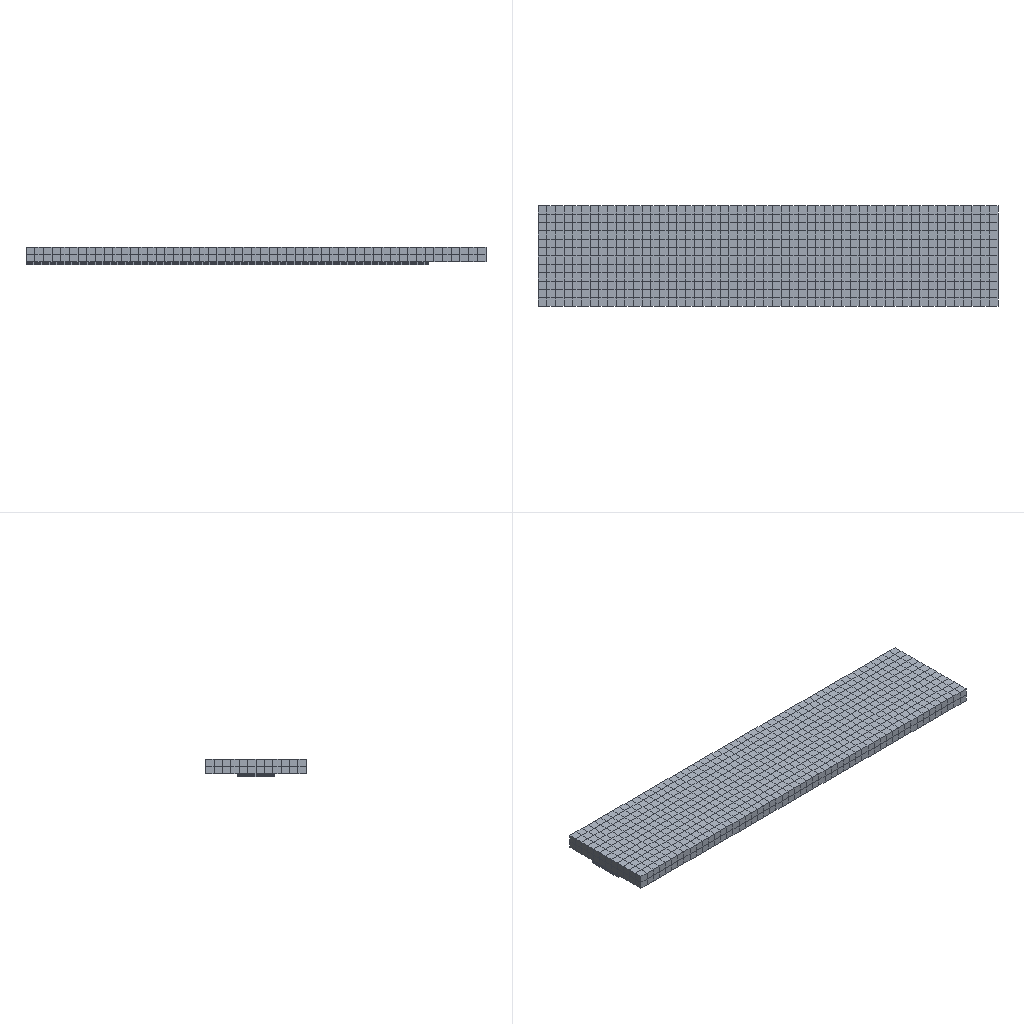Simulation study | abaqus
Set-up summary:
category,name,step,type,value,unit,region
solver,abaqus
solver,version,,,Abaqus/Standard 3DEXPERIENCE R2017x
units,not stated in the deck,,not stated
analysis,deck,,coupled temperature-displacement,coupled temperature-displacement
load_step,Step-1,Step-1,coupled temperature-displacement
load_step,Step-2,Step-2,coupled temperature-displacement
load_step,Step-3,Step-3,coupled temperature-displacement
load_step,Step-4,Step-4,coupled temperature-displacement
load_step,Step-5,Step-5,coupled temperature-displacement
load_step,Step-6,Step-6,coupled temperature-displacement
load_step,Step-7,Step-7,coupled temperature-displacement
load_step,Step-8,Step-8,coupled temperature-displacement
load_step,Step-9,Step-9,coupled temperature-displacement
load_step,Step-10,Step-10,coupled temperature-displacement
load_step,Step-11,Step-11,coupled temperature-displacement
load_step,Step-12,Step-12,coupled temperature-displacement
load_step,Step-13,Step-13,coupled temperature-displacement
load_step,Step-14,Step-14,coupled temperature-displacement
load_step,Step-15,Step-15,coupled temperature-displacement
load_step,Step-16,Step-16,coupled temperature-displacement
load_step,Step-17,Step-17,coupled temperature-displacement
load_step,requested,,,17
mesh,nodes,,,10058
mesh,elements,,,4632
element_type,C3D8T,,solid,4632
load,load commands in deck,,count,19
bc,support commands in deck,,count,1
material,AL,,in results
material,MATERIAL-1,,in results
check,setup vs results,,match,"per instance, exact: element labels, types and connectivity; labels of the nodes the elements use; coordinates of those nodes at SINGLE_PRECISION in 2 of 9 instance(s)"
Abaqus input file, long lists of numbers shortened:
*Heading
** Job name: Job-1 Model name: Model-1-Copy
** Generated by: Abaqus/CAE 2017
*Preprint, echo=NO, model=NO, history=NO, contact=NO
**
** PARTS
**
*Part, name=Part-1
*Node
      1,           0.,         -35.,           5.
      2,           0.,  -32.083,           5.
** (2104 more lines like these left out)
*Element, type=C3D8T
   1,   40,   41,   54,   53,    1,    2,   15,   14
   2,   41,   42,   55,   54,    2,    3,   16,   15
** (1270 more lines like these left out)
*Nset, nset=Set-4, generate
    1,  2106,     1
*Elset, elset=Set-4, generate
    1,  1272,     1
** Section: al
*Solid Section, elset=Set-4, material=al
,
*End Part
**
*Part, name=add
*Node
      1,   30.751,         -10.,           0.
      2,   30.751,         -10.,        0.125
** (992 more lines like these left out)
*Element, type=C3D8T
  1, 161, 166, 485, 315,   1,   2,  17,  84
  2, 315, 485, 486, 316,  84,  17,  18,  83
** (418 more lines like these left out)
*Nset, nset=Set-1, generate
   1,  994,    1
*Elset, elset=Set-1, generate
   1,  420,    1
*Orientation, name=Ori-1
1., 0., 0., 0., 1., 0.
1, 0.
** Section: com
*Solid Section, elset=Set-1, orientation=Ori-1, material=Material-1
,
*End Part
**
**
** ASSEMBLY
**
*Assembly, name=Assembly
**
*Instance, name=Part-1-1, part=Part-1
*End Instance
**
*Instance, name=add-1, part=add
         80.,     6.901,       -0.125
         80.,     6.901,       -0.125,          80.,     6.901,       -1.125,          90.
*End Instance
**
*Instance, name=add-1-lin-2-1, part=add
         80.,     6.901,        -0.25
         80.,     6.901,        -0.25,          80.,     6.901,        -1.25,          90.
*End Instance
**
*Instance, name=add-1-lin-3-1, part=add
         80.,     6.901,       -0.375
         80.,     6.901,       -0.375,          80.,     6.901,       -1.375,          90.
*End Instance
**
*Instance, name=add-1-lin-4-1, part=add
         80.,     6.901,         -0.5
         80.,     6.901,         -0.5,          80.,     6.901,         -1.5,          90.
*End Instance
**
*Instance, name=add-1-lin-5-1, part=add
         80.,     6.901,       -0.625
         80.,     6.901,       -0.625,          80.,     6.901,       -1.625,          90.
*End Instance
**
*Instance, name=add-1-lin-6-1, part=add
         80.,     6.901,        -0.75
         80.,     6.901,        -0.75,          80.,     6.901,        -1.75,          90.
*End Instance
**
*Instance, name=add-1-lin-7-1, part=add
         80.,     6.901,       -0.875
         80.,     6.901,       -0.875,          80.,     6.901,       -1.875,          90.
*End Instance
**
*Instance, name=add-1-lin-8-1, part=add
         80.,     6.901,          -1.
         80.,     6.901,          -1.,          80.,     6.901,          -2.,          90.
*End Instance
**
*Node
      1,           0.,        -17.5,       -0.125
*Node
      2,           0.,        -17.5,       -0.375
*Node
      3,           0.,        -17.5,       -0.625
*Node
      4,           0.,        -17.5,       -0.875
*Node
      5,         140.,        -17.5,        -0.25
*Node
      6,         140.,        -17.5,         -0.5
*Node
      7,         140.,        -17.5,        -0.75
*Nset, nset=Set-10, instance=Part-1-1, generate
 2068,  2106,     1
*Elset, elset=Set-10, instance=Part-1-1, generate
 1249,  1272,     1
*Nset, nset=Set-11, instance=Part-1-1
    1,    2,    3,    4,    5,    6,    7,    8,    9,   10,   11,   12,   13,   14,   15,   16
   17,   18,   19,   20,   21,   22,   23,   24,   25,   26,   27,   28,   29,   30,   31,   32
** (3 more lines like these left out)
*Elset, elset=Set-11, instance=Part-1-1
    1,    2,    3,    4,    5,    6,    7,    8,    9,   10,   11,   12,   13,   14,   15,   16
   17,   18,   19,   20,   21,   22,   23,   24, 1249, 1250, 1251, 1252, 1253, 1254, 1255, 1256
** (1 more lines like these left out)
*Nset, nset=Set-12, instance=Part-1-1, generate
    1,  2106,     1
*Nset, nset=Set-12, instance=add-1, generate
   1,  994,    1
*Nset, nset=Set-12, instance=add-1-lin-2-1, generate
   1,  994,    1
*Nset, nset=Set-12, instance=add-1-lin-6-1, generate
   1,  994,    1
*Nset, nset=Set-12, instance=add-1-lin-4-1, generate
   1,  994,    1
*Nset, nset=Set-12, instance=add-1-lin-8-1, generate
   1,  994,    1
*Nset, nset=Set-12, instance=add-1-lin-3-1, generate
   1,  994,    1
*Nset, nset=Set-12, instance=add-1-lin-7-1, generate
   1,  994,    1
*Nset, nset=Set-12, instance=add-1-lin-5-1, generate
   1,  994,    1
*Elset, elset=Set-12, instance=Part-1-1, generate
    1,  1272,     1
*Elset, elset=Set-12, instance=add-1, generate
   1,  420,    1
*Elset, elset=Set-12, instance=add-1-lin-2-1, generate
   1,  420,    1
*Elset, elset=Set-12, instance=add-1-lin-6-1, generate
   1,  420,    1
*Elset, elset=Set-12, instance=add-1-lin-4-1, generate
   1,  420,    1
*Elset, elset=Set-12, instance=add-1-lin-8-1, generate
   1,  420,    1
*Elset, elset=Set-12, instance=add-1-lin-3-1, generate
   1,  420,    1
*Elset, elset=Set-12, instance=add-1-lin-7-1, generate
   1,  420,    1
*Elset, elset=Set-12, instance=add-1-lin-5-1, generate
   1,  420,    1
*Nset, nset=Set-13, instance=Part-1-1, generate
    1,  2106,     1
*Nset, nset=Set-13, instance=add-1, generate
   1,  994,    1
*Nset, nset=Set-13, instance=add-1-lin-2-1, generate
   1,  994,    1
*Nset, nset=Set-13, instance=add-1-lin-6-1, generate
   1,  994,    1
*Nset, nset=Set-13, instance=add-1-lin-4-1, generate
   1,  994,    1
*Nset, nset=Set-13, instance=add-1-lin-8-1, generate
   1,  994,    1
*Nset, nset=Set-13, instance=add-1-lin-3-1, generate
   1,  994,    1
*Nset, nset=Set-13, instance=add-1-lin-7-1, generate
   1,  994,    1
*Nset, nset=Set-13, instance=add-1-lin-5-1, generate
   1,  994,    1
*Elset, elset=Set-13, instance=Part-1-1, generate
    1,  1272,     1
*Elset, elset=Set-13, instance=add-1, generate
   1,  420,    1
*Elset, elset=Set-13, instance=add-1-lin-2-1, generate
   1,  420,    1
*Elset, elset=Set-13, instance=add-1-lin-6-1, generate
   1,  420,    1
*Elset, elset=Set-13, instance=add-1-lin-4-1, generate
   1,  420,    1
*Elset, elset=Set-13, instance=add-1-lin-8-1, generate
   1,  420,    1
*Elset, elset=Set-13, instance=add-1-lin-3-1, generate
   1,  420,    1
*Elset, elset=Set-13, instance=add-1-lin-7-1, generate
   1,  420,    1
*Elset, elset=Set-13, instance=add-1-lin-5-1, generate
   1,  420,    1
*Nset, nset=Set-14, instance=add-1, generate
   1,  994,    1
*Nset, nset=Set-14, instance=add-1-lin-2-1, generate
   1,  994,    1
*Nset, nset=Set-14, instance=add-1-lin-4-1, generate
   1,  994,    1
*Nset, nset=Set-14, instance=add-1-lin-6-1, generate
   1,  994,    1
*Nset, nset=Set-14, instance=add-1-lin-8-1, generate
   1,  994,    1
*Nset, nset=Set-14, instance=add-1-lin-3-1, generate
   1,  994,    1
*Nset, nset=Set-14, instance=add-1-lin-7-1, generate
   1,  994,    1
*Nset, nset=Set-14, instance=add-1-lin-5-1, generate
   1,  994,    1
*Elset, elset=Set-14, instance=add-1, generate
   1,  420,    1
*Elset, elset=Set-14, instance=add-1-lin-2-1, generate
   1,  420,    1
*Elset, elset=Set-14, instance=add-1-lin-4-1, generate
   1,  420,    1
*Elset, elset=Set-14, instance=add-1-lin-6-1, generate
   1,  420,    1
*Elset, elset=Set-14, instance=add-1-lin-8-1, generate
   1,  420,    1
*Elset, elset=Set-14, instance=add-1-lin-3-1, generate
   1,  420,    1
*Elset, elset=Set-14, instance=add-1-lin-7-1, generate
   1,  420,    1
*Elset, elset=Set-14, instance=add-1-lin-5-1, generate
   1,  420,    1
*Nset, nset=Set-15, instance=add-1, generate
   1,  994,    1
*Elset, elset=Set-15, instance=add-1, generate
   1,  420,    1
*Nset, nset=Set-16, instance=add-1-lin-2-1, generate
   1,  994,    1
*Elset, elset=Set-16, instance=add-1-lin-2-1, generate
   1,  420,    1
*Nset, nset=Set-17, instance=add-1-lin-3-1, generate
   1,  994,    1
*Elset, elset=Set-17, instance=add-1-lin-3-1, generate
   1,  420,    1
*Nset, nset=Set-18, instance=add-1-lin-4-1, generate
   1,  994,    1
*Elset, elset=Set-18, instance=add-1-lin-4-1, generate
   1,  420,    1
*Nset, nset=Set-19, instance=add-1-lin-5-1, generate
   1,  994,    1
*Elset, elset=Set-19, instance=add-1-lin-5-1, generate
   1,  420,    1
*Nset, nset=Set-20, instance=add-1-lin-6-1, generate
   1,  994,    1
*Elset, elset=Set-20, instance=add-1-lin-6-1, generate
   1,  420,    1
*Nset, nset=Set-21, instance=add-1-lin-7-1, generate
   1,  994,    1
*Elset, elset=Set-21, instance=add-1-lin-7-1, generate
   1,  420,    1
*Nset, nset=Set-22, instance=add-1-lin-8-1, generate
   1,  994,    1
*Elset, elset=Set-22, instance=add-1-lin-8-1, generate
   1,  420,    1
*Nset, nset=Set-23, instance=add-1, generate
   1,  994,    1
*Nset, nset=Set-23, instance=add-1-lin-2-1, generate
   1,  994,    1
*Nset, nset=Set-23, instance=add-1-lin-4-1, generate
   1,  994,    1
*Nset, nset=Set-23, instance=add-1-lin-6-1, generate
   1,  994,    1
*Nset, nset=Set-23, instance=add-1-lin-8-1, generate
   1,  994,    1
*Nset, nset=Set-23, instance=add-1-lin-3-1, generate
   1,  994,    1
*Nset, nset=Set-23, instance=add-1-lin-7-1, generate
   1,  994,    1
*Nset, nset=Set-23, instance=add-1-lin-5-1, generate
   1,  994,    1
*Elset, elset=Set-23, instance=add-1, generate
   1,  420,    1
*Elset, elset=Set-23, instance=add-1-lin-2-1, generate
   1,  420,    1
*Elset, elset=Set-23, instance=add-1-lin-4-1, generate
   1,  420,    1
*Elset, elset=Set-23, instance=add-1-lin-6-1, generate
   1,  420,    1
*Elset, elset=Set-23, instance=add-1-lin-8-1, generate
   1,  420,    1
*Elset, elset=Set-23, instance=add-1-lin-3-1, generate
   1,  420,    1
*Elset, elset=Set-23, instance=add-1-lin-7-1, generate
   1,  420,    1
*Elset, elset=Set-23, instance=add-1-lin-5-1, generate
   1,  420,    1
*Elset, elset=_Surf-17_S6, internal, instance=add-1, generate
   1,  210,    1
*Surface, type=ELEMENT, name=Surf-17
_Surf-17_S6, S6
*Elset, elset=_Surf-18_S4, internal, instance=add-1, generate
 211,  420,    1
*Surface, type=ELEMENT, name=Surf-18
_Surf-18_S4, S4
*Elset, elset=_Surf-19_S6, internal, instance=add-1-lin-2-1, generate
   1,  210,    1
*Surface, type=ELEMENT, name=Surf-19
_Surf-19_S6, S6
*Elset, elset=_Surf-20_S4, internal, instance=add-1-lin-2-1, generate
 211,  420,    1
*Surface, type=ELEMENT, name=Surf-20
_Surf-20_S4, S4
*Elset, elset=_Surf-21_S4, internal, instance=add-1-lin-2-1, generate
 211,  420,    1
*Surface, type=ELEMENT, name=Surf-21
_Surf-21_S4, S4
*Elset, elset=_Surf-22_S6, internal, instance=add-1-lin-2-1, generate
   1,  210,    1
*Surface, type=ELEMENT, name=Surf-22
_Surf-22_S6, S6
*Elset, elset=_Surf-23_S6, internal, instance=add-1-lin-3-1, generate
   1,  210,    1
*Surface, type=ELEMENT, name=Surf-23
_Surf-23_S6, S6
*Elset, elset=_Surf-24_S4, internal, instance=add-1-lin-3-1, generate
 211,  420,    1
*Surface, type=ELEMENT, name=Surf-24
_Surf-24_S4, S4
*Elset, elset=_Surf-25_S6, internal, instance=add-1-lin-4-1, generate
   1,  210,    1
*Surface, type=ELEMENT, name=Surf-25
_Surf-25_S6, S6
*Elset, elset=_Surf-26_S4, internal, instance=add-1-lin-4-1, generate
 211,  420,    1
*Surface, type=ELEMENT, name=Surf-26
_Surf-26_S4, S4
*Elset, elset=_Surf-27_S6, internal, instance=add-1-lin-4-1, generate
   1,  210,    1
*Surface, type=ELEMENT, name=Surf-27
_Surf-27_S6, S6
*Elset, elset=_Surf-28_S6, internal, instance=add-1-lin-5-1, generate
   1,  210,    1
*Surface, type=ELEMENT, name=Surf-28
_Surf-28_S6, S6
*Elset, elset=_Surf-29_S4, internal, instance=add-1-lin-5-1, generate
 211,  420,    1
*Surface, type=ELEMENT, name=Surf-29
_Surf-29_S4, S4
*Elset, elset=_Surf-30_S4, internal, instance=add-1-lin-6-1, generate
 211,  420,    1
*Surface, type=ELEMENT, name=Surf-30
_Surf-30_S4, S4
*Elset, elset=_Surf-31_S6, internal, instance=add-1-lin-6-1, generate
   1,  210,    1
*Surface, type=ELEMENT, name=Surf-31
_Surf-31_S6, S6
*Elset, elset=_Surf-32_S6, internal, instance=add-1-lin-7-1, generate
   1,  210,    1
*Surface, type=ELEMENT, name=Surf-32
_Surf-32_S6, S6
*Elset, elset=_Surf-33_S4, internal, instance=add-1-lin-7-1, generate
 211,  420,    1
*Surface, type=ELEMENT, name=Surf-33
_Surf-33_S4, S4
*Elset, elset=_Surf-34_S4, internal, instance=add-1-lin-8-1, generate
 211,  420,    1
*Surface, type=ELEMENT, name=Surf-34
_Surf-34_S4, S4
*Elset, elset=_Surf-35_S6, internal, instance=add-1-lin-8-1, generate
   1,  210,    1
*Surface, type=ELEMENT, name=Surf-35
_Surf-35_S6, S6
*Elset, elset=_Surf-36_S1, internal, instance=Part-1-1, generate
 1249,  1272,     1
*Elset, elset=_Surf-36_S1, internal, instance=add-1, generate
 176,  210,    1
*Elset, elset=_Surf-36_S1, internal, instance=add-1-lin-2-1, generate
 176,  210,    1
*Elset, elset=_Surf-36_S1, internal, instance=add-1-lin-6-1, generate
 176,  210,    1
*Elset, elset=_Surf-36_S1, internal, instance=add-1-lin-4-1, generate
 176,  210,    1
*Elset, elset=_Surf-36_S1, internal, instance=add-1-lin-8-1, generate
 176,  210,    1
*Elset, elset=_Surf-36_S1, internal, instance=add-1-lin-3-1, generate
 176,  210,    1
*Elset, elset=_Surf-36_S1, internal, instance=add-1-lin-7-1, generate
 176,  210,    1
*Elset, elset=_Surf-36_S1, internal, instance=add-1-lin-5-1, generate
 176,  210,    1
*Elset, elset=_Surf-36_S6, internal, instance=Part-1-1, generate
    1,  1261,    12
*Elset, elset=_Surf-36_S6, internal, instance=add-1, generate
   1,  420,    1
*Elset, elset=_Surf-36_S6, internal, instance=add-1-lin-2-1, generate
   1,  420,    1
*Elset, elset=_Surf-36_S6, internal, instance=add-1-lin-6-1, generate
   1,  420,    1
*Elset, elset=_Surf-36_S6, internal, instance=add-1-lin-4-1, generate
   1,  420,    1
*Elset, elset=_Surf-36_S6, internal, instance=add-1-lin-8-1, generate
   1,  420,    1
*Elset, elset=_Surf-36_S6, internal, instance=add-1-lin-3-1, generate
   1,  420,    1
*Elset, elset=_Surf-36_S6, internal, instance=add-1-lin-7-1, generate
   1,  420,    1
*Elset, elset=_Surf-36_S6, internal, instance=add-1-lin-5-1, generate
   1,  420,    1
*Elset, elset=_Surf-36_S2, internal, instance=Part-1-1, generate
  1,  24,   1
*Elset, elset=_Surf-36_S2, internal, instance=add-1
   1,   2,   3,   4,   5,   6,   7,   8,   9,  10,  11,  12,  13,  14,  15,  16
  17,  18,  19,  20,  21,  22,  23,  24,  25,  26,  27,  28,  29,  30,  31,  32
** (1 more lines like these left out)
*Elset, elset=_Surf-36_S2, internal, instance=add-1-lin-2-1
   1,   2,   3,   4,   5,   6,   7,   8,   9,  10,  11,  12,  13,  14,  15,  16
  17,  18,  19,  20,  21,  22,  23,  24,  25,  26,  27,  28,  29,  30,  31,  32
** (1 more lines like these left out)
*Elset, elset=_Surf-36_S2, internal, instance=add-1-lin-6-1
   1,   2,   3,   4,   5,   6,   7,   8,   9,  10,  11,  12,  13,  14,  15,  16
  17,  18,  19,  20,  21,  22,  23,  24,  25,  26,  27,  28,  29,  30,  31,  32
** (1 more lines like these left out)
*Elset, elset=_Surf-36_S2, internal, instance=add-1-lin-4-1
   1,   2,   3,   4,   5,   6,   7,   8,   9,  10,  11,  12,  13,  14,  15,  16
  17,  18,  19,  20,  21,  22,  23,  24,  25,  26,  27,  28,  29,  30,  31,  32
** (1 more lines like these left out)
*Elset, elset=_Surf-36_S2, internal, instance=add-1-lin-8-1
   1,   2,   3,   4,   5,   6,   7,   8,   9,  10,  11,  12,  13,  14,  15,  16
  17,  18,  19,  20,  21,  22,  23,  24,  25,  26,  27,  28,  29,  30,  31,  32
** (1 more lines like these left out)
*Elset, elset=_Surf-36_S2, internal, instance=add-1-lin-3-1
   1,   2,   3,   4,   5,   6,   7,   8,   9,  10,  11,  12,  13,  14,  15,  16
  17,  18,  19,  20,  21,  22,  23,  24,  25,  26,  27,  28,  29,  30,  31,  32
** (1 more lines like these left out)
*Elset, elset=_Surf-36_S2, internal, instance=add-1-lin-7-1
   1,   2,   3,   4,   5,   6,   7,   8,   9,  10,  11,  12,  13,  14,  15,  16
  17,  18,  19,  20,  21,  22,  23,  24,  25,  26,  27,  28,  29,  30,  31,  32
** (1 more lines like these left out)
*Elset, elset=_Surf-36_S2, internal, instance=add-1-lin-5-1
   1,   2,   3,   4,   5,   6,   7,   8,   9,  10,  11,  12,  13,  14,  15,  16
  17,  18,  19,  20,  21,  22,  23,  24,  25,  26,  27,  28,  29,  30,  31,  32
** (1 more lines like these left out)
*Elset, elset=_Surf-36_S4, internal, instance=Part-1-1, generate
   12,  1272,    12
*Elset, elset=_Surf-36_S4, internal, instance=add-1, generate
   1,  420,    1
*Elset, elset=_Surf-36_S4, internal, instance=add-1-lin-2-1, generate
   1,  420,    1
*Elset, elset=_Surf-36_S4, internal, instance=add-1-lin-6-1, generate
   1,  420,    1
*Elset, elset=_Surf-36_S4, internal, instance=add-1-lin-4-1, generate
   1,  420,    1
*Elset, elset=_Surf-36_S4, internal, instance=add-1-lin-8-1, generate
   1,  420,    1
*Elset, elset=_Surf-36_S4, internal, instance=add-1-lin-3-1, generate
   1,  420,    1
*Elset, elset=_Surf-36_S4, internal, instance=add-1-lin-7-1, generate
   1,  420,    1
*Elset, elset=_Surf-36_S4, internal, instance=add-1-lin-5-1, generate
   1,  420,    1
*Elset, elset=_Surf-36_S3, internal, instance=Part-1-1
    1,    2,    3,    4,    5,    6,    7,    8,    9,   10,   11,   12,   25,   26,   27,   28
   29,   30,   31,   32,   33,   34,   35,   36,   49,   50,   51,   52,   53,   54,   55,   56
** (38 more lines like these left out)
*Elset, elset=_Surf-36_S3, internal, instance=add-1, generate
 211,  415,    6
*Elset, elset=_Surf-36_S3, internal, instance=add-1-lin-2-1, generate
 211,  415,    6
*Elset, elset=_Surf-36_S3, internal, instance=add-1-lin-6-1, generate
 211,  415,    6
*Elset, elset=_Surf-36_S3, internal, instance=add-1-lin-4-1, generate
 211,  415,    6
*Elset, elset=_Surf-36_S3, internal, instance=add-1-lin-8-1, generate
 211,  415,    6
*Elset, elset=_Surf-36_S3, internal, instance=add-1-lin-3-1, generate
 211,  415,    6
*Elset, elset=_Surf-36_S3, internal, instance=add-1-lin-7-1, generate
 211,  415,    6
*Elset, elset=_Surf-36_S3, internal, instance=add-1-lin-5-1, generate
 211,  415,    6
*Elset, elset=_Surf-36_S5, internal, instance=Part-1-1
   13,   14,   15,   16,   17,   18,   19,   20,   21,   22,   23,   24,   37,   38,   39,   40
   41,   42,   43,   44,   45,   46,   47,   48,   61,   62,   63,   64,   65,   66,   67,   68
** (38 more lines like these left out)
*Elset, elset=_Surf-36_S5, internal, instance=add-1
  35,  70, 105, 140, 175, 210, 216, 222, 228, 234, 240, 246, 252, 258, 264, 270
 276, 282, 288, 294, 300, 306, 312, 318, 324, 330, 336, 342, 348, 354, 360, 366
** (1 more lines like these left out)
*Elset, elset=_Surf-36_S5, internal, instance=add-1-lin-2-1
  35,  70, 105, 140, 175, 210, 216, 222, 228, 234, 240, 246, 252, 258, 264, 270
 276, 282, 288, 294, 300, 306, 312, 318, 324, 330, 336, 342, 348, 354, 360, 366
** (1 more lines like these left out)
*Elset, elset=_Surf-36_S5, internal, instance=add-1-lin-6-1
  35,  70, 105, 140, 175, 210, 216, 222, 228, 234, 240, 246, 252, 258, 264, 270
 276, 282, 288, 294, 300, 306, 312, 318, 324, 330, 336, 342, 348, 354, 360, 366
** (1 more lines like these left out)
*Elset, elset=_Surf-36_S5, internal, instance=add-1-lin-4-1
  35,  70, 105, 140, 175, 210, 216, 222, 228, 234, 240, 246, 252, 258, 264, 270
 276, 282, 288, 294, 300, 306, 312, 318, 324, 330, 336, 342, 348, 354, 360, 366
** (1 more lines like these left out)
*Elset, elset=_Surf-36_S5, internal, instance=add-1-lin-8-1
  35,  70, 105, 140, 175, 210, 216, 222, 228, 234, 240, 246, 252, 258, 264, 270
 276, 282, 288, 294, 300, 306, 312, 318, 324, 330, 336, 342, 348, 354, 360, 366
** (1 more lines like these left out)
*Elset, elset=_Surf-36_S5, internal, instance=add-1-lin-3-1
  35,  70, 105, 140, 175, 210, 216, 222, 228, 234, 240, 246, 252, 258, 264, 270
 276, 282, 288, 294, 300, 306, 312, 318, 324, 330, 336, 342, 348, 354, 360, 366
** (1 more lines like these left out)
*Elset, elset=_Surf-36_S5, internal, instance=add-1-lin-7-1
  35,  70, 105, 140, 175, 210, 216, 222, 228, 234, 240, 246, 252, 258, 264, 270
 276, 282, 288, 294, 300, 306, 312, 318, 324, 330, 336, 342, 348, 354, 360, 366
** (1 more lines like these left out)
*Elset, elset=_Surf-36_S5, internal, instance=add-1-lin-5-1
  35,  70, 105, 140, 175, 210, 216, 222, 228, 234, 240, 246, 252, 258, 264, 270
 276, 282, 288, 294, 300, 306, 312, 318, 324, 330, 336, 342, 348, 354, 360, 366
** (1 more lines like these left out)
*Surface, type=ELEMENT, name=Surf-36
_Surf-36_S1, S1
_Surf-36_S6, S6
_Surf-36_S2, S2
_Surf-36_S4, S4
_Surf-36_S3, S3
_Surf-36_S5, S5
*Elset, elset=_Surf-37_S1, internal, instance=Part-1-1, generate
 1249,  1272,     1
*Elset, elset=_Surf-37_S1, internal, instance=add-1, generate
 176,  210,    1
*Elset, elset=_Surf-37_S1, internal, instance=add-1-lin-2-1, generate
 176,  210,    1
*Elset, elset=_Surf-37_S1, internal, instance=add-1-lin-6-1, generate
 176,  210,    1
*Elset, elset=_Surf-37_S1, internal, instance=add-1-lin-4-1, generate
 176,  210,    1
*Elset, elset=_Surf-37_S1, internal, instance=add-1-lin-8-1, generate
 176,  210,    1
*Elset, elset=_Surf-37_S1, internal, instance=add-1-lin-3-1, generate
 176,  210,    1
*Elset, elset=_Surf-37_S1, internal, instance=add-1-lin-7-1, generate
 176,  210,    1
*Elset, elset=_Surf-37_S1, internal, instance=add-1-lin-5-1, generate
 176,  210,    1
*Elset, elset=_Surf-37_S6, internal, instance=Part-1-1, generate
    1,  1261,    12
*Elset, elset=_Surf-37_S6, internal, instance=add-1, generate
   1,  420,    1
*Elset, elset=_Surf-37_S6, internal, instance=add-1-lin-2-1, generate
   1,  420,    1
*Elset, elset=_Surf-37_S6, internal, instance=add-1-lin-6-1, generate
   1,  420,    1
*Elset, elset=_Surf-37_S6, internal, instance=add-1-lin-4-1, generate
   1,  420,    1
*Elset, elset=_Surf-37_S6, internal, instance=add-1-lin-8-1, generate
   1,  420,    1
*Elset, elset=_Surf-37_S6, internal, instance=add-1-lin-3-1, generate
   1,  420,    1
*Elset, elset=_Surf-37_S6, internal, instance=add-1-lin-7-1, generate
   1,  420,    1
*Elset, elset=_Surf-37_S6, internal, instance=add-1-lin-5-1, generate
   1,  420,    1
*Elset, elset=_Surf-37_S2, internal, instance=Part-1-1, generate
  1,  24,   1
*Elset, elset=_Surf-37_S2, internal, instance=add-1
   1,   2,   3,   4,   5,   6,   7,   8,   9,  10,  11,  12,  13,  14,  15,  16
  17,  18,  19,  20,  21,  22,  23,  24,  25,  26,  27,  28,  29,  30,  31,  32
** (1 more lines like these left out)
*Elset, elset=_Surf-37_S2, internal, instance=add-1-lin-2-1
   1,   2,   3,   4,   5,   6,   7,   8,   9,  10,  11,  12,  13,  14,  15,  16
  17,  18,  19,  20,  21,  22,  23,  24,  25,  26,  27,  28,  29,  30,  31,  32
** (1 more lines like these left out)
*Elset, elset=_Surf-37_S2, internal, instance=add-1-lin-6-1
   1,   2,   3,   4,   5,   6,   7,   8,   9,  10,  11,  12,  13,  14,  15,  16
  17,  18,  19,  20,  21,  22,  23,  24,  25,  26,  27,  28,  29,  30,  31,  32
** (1 more lines like these left out)
*Elset, elset=_Surf-37_S2, internal, instance=add-1-lin-4-1
   1,   2,   3,   4,   5,   6,   7,   8,   9,  10,  11,  12,  13,  14,  15,  16
  17,  18,  19,  20,  21,  22,  23,  24,  25,  26,  27,  28,  29,  30,  31,  32
** (1 more lines like these left out)
*Elset, elset=_Surf-37_S2, internal, instance=add-1-lin-8-1
   1,   2,   3,   4,   5,   6,   7,   8,   9,  10,  11,  12,  13,  14,  15,  16
  17,  18,  19,  20,  21,  22,  23,  24,  25,  26,  27,  28,  29,  30,  31,  32
** (1 more lines like these left out)
*Elset, elset=_Surf-37_S2, internal, instance=add-1-lin-3-1
   1,   2,   3,   4,   5,   6,   7,   8,   9,  10,  11,  12,  13,  14,  15,  16
  17,  18,  19,  20,  21,  22,  23,  24,  25,  26,  27,  28,  29,  30,  31,  32
** (1 more lines like these left out)
*Elset, elset=_Surf-37_S2, internal, instance=add-1-lin-7-1
   1,   2,   3,   4,   5,   6,   7,   8,   9,  10,  11,  12,  13,  14,  15,  16
  17,  18,  19,  20,  21,  22,  23,  24,  25,  26,  27,  28,  29,  30,  31,  32
** (1 more lines like these left out)
*Elset, elset=_Surf-37_S2, internal, instance=add-1-lin-5-1
   1,   2,   3,   4,   5,   6,   7,   8,   9,  10,  11,  12,  13,  14,  15,  16
  17,  18,  19,  20,  21,  22,  23,  24,  25,  26,  27,  28,  29,  30,  31,  32
** (1 more lines like these left out)
*Elset, elset=_Surf-37_S4, internal, instance=Part-1-1, generate
   12,  1272,    12
*Elset, elset=_Surf-37_S4, internal, instance=add-1, generate
   1,  420,    1
*Elset, elset=_Surf-37_S4, internal, instance=add-1-lin-2-1, generate
   1,  420,    1
*Elset, elset=_Surf-37_S4, internal, instance=add-1-lin-6-1, generate
   1,  420,    1
*Elset, elset=_Surf-37_S4, internal, instance=add-1-lin-4-1, generate
   1,  420,    1
*Elset, elset=_Surf-37_S4, internal, instance=add-1-lin-8-1, generate
   1,  420,    1
*Elset, elset=_Surf-37_S4, internal, instance=add-1-lin-3-1, generate
   1,  420,    1
*Elset, elset=_Surf-37_S4, internal, instance=add-1-lin-7-1, generate
   1,  420,    1
*Elset, elset=_Surf-37_S4, internal, instance=add-1-lin-5-1, generate
   1,  420,    1
*Elset, elset=_Surf-37_S3, internal, instance=Part-1-1
    1,    2,    3,    4,    5,    6,    7,    8,    9,   10,   11,   12,   25,   26,   27,   28
   29,   30,   31,   32,   33,   34,   35,   36,   49,   50,   51,   52,   53,   54,   55,   56
** (38 more lines like these left out)
*Elset, elset=_Surf-37_S3, internal, instance=add-1, generate
 211,  415,    6
*Elset, elset=_Surf-37_S3, internal, instance=add-1-lin-2-1, generate
 211,  415,    6
*Elset, elset=_Surf-37_S3, internal, instance=add-1-lin-6-1, generate
 211,  415,    6
*Elset, elset=_Surf-37_S3, internal, instance=add-1-lin-4-1, generate
 211,  415,    6
*Elset, elset=_Surf-37_S3, internal, instance=add-1-lin-8-1, generate
 211,  415,    6
*Elset, elset=_Surf-37_S3, internal, instance=add-1-lin-3-1, generate
 211,  415,    6
*Elset, elset=_Surf-37_S3, internal, instance=add-1-lin-7-1, generate
 211,  415,    6
*Elset, elset=_Surf-37_S3, internal, instance=add-1-lin-5-1, generate
 211,  415,    6
*Elset, elset=_Surf-37_S5, internal, instance=Part-1-1
   13,   14,   15,   16,   17,   18,   19,   20,   21,   22,   23,   24,   37,   38,   39,   40
   41,   42,   43,   44,   45,   46,   47,   48,   61,   62,   63,   64,   65,   66,   67,   68
** (38 more lines like these left out)
*Elset, elset=_Surf-37_S5, internal, instance=add-1
  35,  70, 105, 140, 175, 210, 216, 222, 228, 234, 240, 246, 252, 258, 264, 270
 276, 282, 288, 294, 300, 306, 312, 318, 324, 330, 336, 342, 348, 354, 360, 366
** (1 more lines like these left out)
*Elset, elset=_Surf-37_S5, internal, instance=add-1-lin-2-1
  35,  70, 105, 140, 175, 210, 216, 222, 228, 234, 240, 246, 252, 258, 264, 270
 276, 282, 288, 294, 300, 306, 312, 318, 324, 330, 336, 342, 348, 354, 360, 366
** (1 more lines like these left out)
*Elset, elset=_Surf-37_S5, internal, instance=add-1-lin-6-1
  35,  70, 105, 140, 175, 210, 216, 222, 228, 234, 240, 246, 252, 258, 264, 270
 276, 282, 288, 294, 300, 306, 312, 318, 324, 330, 336, 342, 348, 354, 360, 366
** (1 more lines like these left out)
*Elset, elset=_Surf-37_S5, internal, instance=add-1-lin-4-1
  35,  70, 105, 140, 175, 210, 216, 222, 228, 234, 240, 246, 252, 258, 264, 270
 276, 282, 288, 294, 300, 306, 312, 318, 324, 330, 336, 342, 348, 354, 360, 366
** (1 more lines like these left out)
*Elset, elset=_Surf-37_S5, internal, instance=add-1-lin-8-1
  35,  70, 105, 140, 175, 210, 216, 222, 228, 234, 240, 246, 252, 258, 264, 270
 276, 282, 288, 294, 300, 306, 312, 318, 324, 330, 336, 342, 348, 354, 360, 366
** (1 more lines like these left out)
*Elset, elset=_Surf-37_S5, internal, instance=add-1-lin-3-1
  35,  70, 105, 140, 175, 210, 216, 222, 228, 234, 240, 246, 252, 258, 264, 270
 276, 282, 288, 294, 300, 306, 312, 318, 324, 330, 336, 342, 348, 354, 360, 366
** (1 more lines like these left out)
*Elset, elset=_Surf-37_S5, internal, instance=add-1-lin-7-1
  35,  70, 105, 140, 175, 210, 216, 222, 228, 234, 240, 246, 252, 258, 264, 270
 276, 282, 288, 294, 300, 306, 312, 318, 324, 330, 336, 342, 348, 354, 360, 366
** (1 more lines like these left out)
*Elset, elset=_Surf-37_S5, internal, instance=add-1-lin-5-1
  35,  70, 105, 140, 175, 210, 216, 222, 228, 234, 240, 246, 252, 258, 264, 270
 276, 282, 288, 294, 300, 306, 312, 318, 324, 330, 336, 342, 348, 354, 360, 366
** (1 more lines like these left out)
*Surface, type=ELEMENT, name=Surf-37
_Surf-37_S1, S1
_Surf-37_S6, S6
_Surf-37_S2, S2
_Surf-37_S4, S4
_Surf-37_S3, S3
_Surf-37_S5, S5
*Elset, elset=_m_Surf-1_S6, internal, instance=add-1, generate
 211,  420,    1
*Elset, elset=_m_Surf-1_S4, internal, instance=add-1, generate
   1,  210,    1
*Surface, type=ELEMENT, name=m_Surf-1
_m_Surf-1_S6, S6
_m_Surf-1_S4, S4
*Elset, elset=_m_Surf-3_S6, internal, instance=add-1-lin-2-1, generate
 211,  420,    1
*Elset, elset=_m_Surf-3_S4, internal, instance=add-1-lin-2-1, generate
   1,  210,    1
*Surface, type=ELEMENT, name=m_Surf-3
_m_Surf-3_S6, S6
_m_Surf-3_S4, S4
*Elset, elset=_m_Surf-5_S6, internal, instance=add-1-lin-3-1, generate
 211,  420,    1
*Elset, elset=_m_Surf-5_S4, internal, instance=add-1-lin-3-1, generate
   1,  210,    1
*Surface, type=ELEMENT, name=m_Surf-5
_m_Surf-5_S6, S6
_m_Surf-5_S4, S4
*Elset, elset=_m_Surf-7_S6, internal, instance=add-1-lin-4-1, generate
 211,  420,    1
*Elset, elset=_m_Surf-7_S4, internal, instance=add-1-lin-4-1, generate
   1,  210,    1
*Surface, type=ELEMENT, name=m_Surf-7
_m_Surf-7_S6, S6
_m_Surf-7_S4, S4
*Elset, elset=_m_Surf-9_S6, internal, instance=add-1-lin-5-1, generate
 211,  420,    1
*Elset, elset=_m_Surf-9_S4, internal, instance=add-1-lin-5-1, generate
   1,  210,    1
*Surface, type=ELEMENT, name=m_Surf-9
_m_Surf-9_S6, S6
_m_Surf-9_S4, S4
*Elset, elset=_m_Surf-11_S6, internal, instance=add-1-lin-6-1, generate
 211,  420,    1
*Elset, elset=_m_Surf-11_S4, internal, instance=add-1-lin-6-1, generate
   1,  210,    1
*Surface, type=ELEMENT, name=m_Surf-11
_m_Surf-11_S6, S6
_m_Surf-11_S4, S4
*Elset, elset=_m_Surf-13_S6, internal, instance=add-1-lin-7-1, generate
 211,  420,    1
*Elset, elset=_m_Surf-13_S4, internal, instance=add-1-lin-7-1, generate
   1,  210,    1
*Surface, type=ELEMENT, name=m_Surf-13
_m_Surf-13_S6, S6
_m_Surf-13_S4, S4
*Elset, elset=_m_Surf-15_S6, internal, instance=add-1-lin-8-1, generate
 211,  420,    1
*Elset, elset=_m_Surf-15_S4, internal, instance=add-1-lin-8-1, generate
   1,  210,    1
*Surface, type=ELEMENT, name=m_Surf-15
_m_Surf-15_S6, S6
_m_Surf-15_S4, S4
*Elset, elset=_s_Surf-1_S5, internal, instance=Part-1-1
   13,   14,   15,   16,   17,   18,   19,   20,   21,   22,   23,   24,   37,   38,   39,   40
   41,   42,   43,   44,   45,   46,   47,   48,   61,   62,   63,   64,   65,   66,   67,   68
** (38 more lines like these left out)
*Surface, type=ELEMENT, name=s_Surf-1
_s_Surf-1_S5, S5
*Elset, elset=_s_Surf-3_S6, internal, instance=add-1, generate
   1,  210,    1
*Elset, elset=_s_Surf-3_S4, internal, instance=add-1, generate
 211,  420,    1
*Surface, type=ELEMENT, name=s_Surf-3
_s_Surf-3_S6, S6
_s_Surf-3_S4, S4
*Elset, elset=_s_Surf-5_S6, internal, instance=add-1-lin-2-1, generate
   1,  210,    1
*Elset, elset=_s_Surf-5_S4, internal, instance=add-1-lin-2-1, generate
 211,  420,    1
*Surface, type=ELEMENT, name=s_Surf-5
_s_Surf-5_S6, S6
_s_Surf-5_S4, S4
*Elset, elset=_s_Surf-7_S6, internal, instance=add-1-lin-3-1, generate
   1,  210,    1
*Elset, elset=_s_Surf-7_S4, internal, instance=add-1-lin-3-1, generate
 211,  420,    1
*Surface, type=ELEMENT, name=s_Surf-7
_s_Surf-7_S6, S6
_s_Surf-7_S4, S4
*Elset, elset=_s_Surf-9_S6, internal, instance=add-1-lin-4-1, generate
   1,  210,    1
*Elset, elset=_s_Surf-9_S4, internal, instance=add-1-lin-4-1, generate
 211,  420,    1
*Surface, type=ELEMENT, name=s_Surf-9
_s_Surf-9_S6, S6
_s_Surf-9_S4, S4
*Elset, elset=_s_Surf-11_S6, internal, instance=add-1-lin-5-1, generate
   1,  210,    1
*Elset, elset=_s_Surf-11_S4, internal, instance=add-1-lin-5-1, generate
 211,  420,    1
*Surface, type=ELEMENT, name=s_Surf-11
_s_Surf-11_S6, S6
_s_Surf-11_S4, S4
*Elset, elset=_s_Surf-13_S6, internal, instance=add-1-lin-6-1, generate
   1,  210,    1
*Elset, elset=_s_Surf-13_S4, internal, instance=add-1-lin-6-1, generate
 211,  420,    1
*Surface, type=ELEMENT, name=s_Surf-13
_s_Surf-13_S6, S6
_s_Surf-13_S4, S4
*Elset, elset=_s_Surf-15_S6, internal, instance=add-1-lin-7-1, generate
   1,  210,    1
*Elset, elset=_s_Surf-15_S4, internal, instance=add-1-lin-7-1, generate
 211,  420,    1
*Surface, type=ELEMENT, name=s_Surf-15
_s_Surf-15_S6, S6
_s_Surf-15_S4, S4
** Constraint: Constraint-1
*Tie, name=Constraint-1, adjust=yes
m_Surf-1, s_Surf-1
** Constraint: Constraint-2
*Tie, name=Constraint-2, adjust=yes
s_Surf-3, m_Surf-3
** Constraint: Constraint-3
*Tie, name=Constraint-3, adjust=yes
s_Surf-5, m_Surf-5
** Constraint: Constraint-4
*Tie, name=Constraint-4, adjust=yes
s_Surf-7, m_Surf-7
** Constraint: Constraint-5
*Tie, name=Constraint-5, adjust=yes
s_Surf-9, m_Surf-9
** Constraint: Constraint-6
*Tie, name=Constraint-6, adjust=yes
s_Surf-11, m_Surf-11
** Constraint: Constraint-7
*Tie, name=Constraint-7, adjust=yes
s_Surf-13, m_Surf-13
** Constraint: Constraint-8
*Tie, name=Constraint-8, adjust=yes
s_Surf-15, m_Surf-15
*End Assembly
*Amplitude, name=Amp-1
             0.,              1.,             0.5,              1.,            0.51,              0.
*Amplitude, name=Amp-2
           0.51,              0.,           0.511,              1.,              1.,              1.
**
** MATERIALS
**
*Material, name=Material-1
*Conductivity
 3.5,  0.
 4.6, 50.
 5.1,100.
 5.9,150.
 5.9,200.
 6.1,250.
 6.7,300.
 6.8,350.
  7.,400.
*Density
 1.57e-09,
*Elastic, type=ENGINEERING CONSTANTS
130000., 10300.,130000.,   0.25,    0.2,   0.25,  6000.,  6000.
  4800.,    23.
*Expansion
 1e-07,  0.
 3e-07, 50.
 5e-07,100.
 2e-07,150.
    0.,200.
    0.,250.
    0.,300.
    0.,350.
    0.,400.
*Specific Heat
    8e+08,  0.
  9.3e+08, 50.
 1.04e+09,100.
 1.26e+09,150.
  1.3e+09,200.
  1.4e+09,250.
 1.55e+09,300.
 1.65e+09,350.
  1.7e+09,400.
*Material, name=al
*Conductivity
140.,
*Density
 2.78e-09,
*Elastic
72000., 0.3
*Specific Heat
 8.6e+08,
**
** PHYSICAL CONSTANTS
**
*Physical Constants, absolute zero=-273., stefan boltzmann=5.67e-08
**
** BOUNDARY CONDITIONS
**
** Name: BC-1 Type: 对称/反对称/完全固定
*Boundary
Set-11, ENCASTRE
**
** PREDEFINED FIELDS
**
** Name: Predefined Field-1   Type: Temperature
*Initial Conditions, type=TEMPERATURE
Set-13, 20.
** ----------------------------------------------------------------
**
** STEP: Step-1
**
*Step, name=Step-1, nlgeom=YES
*Coupled Temperature-displacement, creep=none, deltmx=1e+06
1e-05, 1e-05, 1e-10, 1e-05
**
** INTERACTIONS
**
** Interaction: Int-del-all
*Model Change, remove
Set-23,
**
** OUTPUT REQUESTS
**
*Restart, write, frequency=0
**
** FIELD OUTPUT: F-Output-1
**
*Output, field, variable=PRESELECT
**
** HISTORY OUTPUT: H-Output-1
**
*Output, history, variable=PRESELECT
*End Step
** ----------------------------------------------------------------
**
** STEP: Step-2
**
*Step, name=Step-2, nlgeom=YES
*Coupled Temperature-displacement, creep=none, deltmx=100000.
0.01, 1., 1e-05, 1.
**
** LOADS
**
** Name: Load-1-1   Type: Pressure
*Dsload, amplitude=Amp-1
Surf-17, P, 0.01
** Name: Load-1-2   Type: Pressure
*Dsload, amplitude=Amp-2
Surf-18, P, 0.01
** Name: Load-17   Type: Body heat flux
*Dflux
Set-14, BFNU, 1.
**
** INTERACTIONS
**
** Interaction: Int-add-1
*Model Change, add
Set-15,
** Interaction: Int-transfer
*Sradiate
Surf-36, R, 20., 0.2
** Interaction: Int-transfer-2
*Sfilm
Surf-37, F, 20., 0.05
**
** OUTPUT REQUESTS
**
*Restart, write, frequency=0
**
** FIELD OUTPUT: F-Output-1
**
*Output, field
*Node Output
CF, NT, RF, RFL, U, V
*Element Output, directions=YES
E, HFL, LE, MISES, MISESMAX, PE, PEEQ, PEMAG, S, TEMP
*Contact Output
CDISP, CSTRESS
**
** HISTORY OUTPUT: H-Output-1
**
*Output, history, variable=PRESELECT
*End Step
** ----------------------------------------------------------------
**
** STEP: Step-3
**
*Step, name=Step-3, nlgeom=YES
*Coupled Temperature-displacement, creep=none, deltmx=100000.
0.01, 1., 1e-05, 1.
**
** OUTPUT REQUESTS
**
*Restart, write, frequency=0
**
** FIELD OUTPUT: F-Output-1
**
*Output, field
*Node Output
CF, NT, RF, RFL, U, V
*Element Output, directions=YES
E, HFL, LE, MISES, MISESMAX, PE, PEEQ, PEMAG, S, TEMP
*Contact Output
CDISP, CSTRESS
**
** HISTORY OUTPUT: H-Output-1
**
*Output, history, variable=PRESELECT
*End Step
** ----------------------------------------------------------------
**
** STEP: Step-4
**
*Step, name=Step-4, nlgeom=YES, inc=1000
*Coupled Temperature-displacement, creep=none, deltmx=10000.
0.01, 1., 1e-05, 1.
**
** LOADS
**
** Name: Load-2-1   Type: Pressure
*Dsload, amplitude=Amp-1
Surf-21, P, 0.01
** Name: Load-2-2   Type: Pressure
*Dsload, amplitude=Amp-2
Surf-22, P, 0.01
**
** INTERACTIONS
**
** Interaction: Int-add-2
*Model Change, add
Set-16,
**
** OUTPUT REQUESTS
**
*Restart, write, frequency=0
**
** FIELD OUTPUT: F-Output-1
**
*Output, field
*Node Output
CF, NT, RF, RFL, U, V
*Element Output, directions=YES
E, HFL, LE, MISES, MISESMAX, PE, PEEQ, PEMAG, S, TEMP
*Contact Output
CDISP, CSTRESS
**
** HISTORY OUTPUT: H-Output-1
**
*Output, history, variable=PRESELECT
*End Step
** ----------------------------------------------------------------
**
** STEP: Step-5
**
*Step, name=Step-5, nlgeom=YES
*Coupled Temperature-displacement, creep=none, deltmx=10000.
0.01, 1., 1e-05, 1.
**
** OUTPUT REQUESTS
**
*Restart, write, frequency=0
**
** FIELD OUTPUT: F-Output-1
**
*Output, field
*Node Output
CF, NT, RF, RFL, U, V
*Element Output, directions=YES
E, HFL, LE, MISES, MISESMAX, PE, PEEQ, PEMAG, S, TEMP
*Contact Output
CDISP, CSTRESS
**
** HISTORY OUTPUT: H-Output-1
**
*Output, history, variable=PRESELECT
*End Step
** ----------------------------------------------------------------
**
** STEP: Step-6
**
*Step, name=Step-6, nlgeom=YES, inc=1000
*Coupled Temperature-displacement, creep=none, deltmx=10000.
0.01, 1., 1e-05, 1.
**
** LOADS
**
** Name: Load-3-1   Type: Pressure
*Dsload, amplitude=Amp-1
Surf-23, P, 0.01
** Name: Load-3-2   Type: Pressure
*Dsload, amplitude=Amp-2
Surf-24, P, 0.01
**
** INTERACTIONS
**
** Interaction: Int-add-3
*Model Change, add
Set-17,
**
** OUTPUT REQUESTS
**
*Restart, write, frequency=0
**
** FIELD OUTPUT: F-Output-1
**
*Output, field
*Node Output
CF, NT, RF, RFL, U, V
*Element Output, directions=YES
E, HFL, LE, MISES, MISESMAX, PE, PEEQ, PEMAG, S, TEMP
*Contact Output
CDISP, CSTRESS
**
** HISTORY OUTPUT: H-Output-1
**
*Output, history, variable=PRESELECT
*End Step
** ----------------------------------------------------------------
**
** STEP: Step-7
**
*Step, name=Step-7, nlgeom=YES, inc=1000
*Coupled Temperature-displacement, creep=none, deltmx=10000.
0.01, 1., 1e-05, 1.
**
** OUTPUT REQUESTS
**
*Restart, write, frequency=0
**
** FIELD OUTPUT: F-Output-1
**
*Output, field
*Node Output
CF, NT, RF, RFL, U, V
*Element Output, directions=YES
E, HFL, LE, MISES, MISESMAX, PE, PEEQ, PEMAG, S, TEMP
*Contact Output
CDISP, CSTRESS
**
** HISTORY OUTPUT: H-Output-1
**
*Output, history, variable=PRESELECT
*End Step
** ----------------------------------------------------------------
**
** STEP: Step-8
**
*Step, name=Step-8, nlgeom=YES
*Coupled Temperature-displacement, creep=none, deltmx=10000.
0.01, 1., 1e-05, 1.
**
** LOADS
**
** Name: Load-4-1   Type: Pressure
*Dsload, amplitude=Amp-1
Surf-26, P, 0.01
** Name: Load-4-2   Type: Pressure
*Dsload, amplitude=Amp-2
Surf-27, P, 0.01
**
** INTERACTIONS
**
** Interaction: Int-add-4
*Model Change, add
Set-18,
**
** OUTPUT REQUESTS
**
*Restart, write, frequency=0
**
** FIELD OUTPUT: F-Output-1
**
*Output, field
*Node Output
CF, NT, RF, RFL, U, V
*Element Output, directions=YES
E, HFL, LE, MISES, MISESMAX, PE, PEEQ, PEMAG, S, TEMP
*Contact Output
CDISP, CSTRESS
**
** HISTORY OUTPUT: H-Output-1
**
*Output, history, variable=PRESELECT
*End Step
** ----------------------------------------------------------------
**
** STEP: Step-9
**
*Step, name=Step-9, nlgeom=YES
*Coupled Temperature-displacement, creep=none, deltmx=10000.
0.01, 1., 1e-05, 1.
**
** OUTPUT REQUESTS
**
*Restart, write, frequency=0
**
** FIELD OUTPUT: F-Output-1
**
*Output, field
*Node Output
CF, NT, RF, RFL, U, V
*Element Output, directions=YES
E, HFL, LE, MISES, MISESMAX, PE, PEEQ, PEMAG, S, TEMP
*Contact Output
CDISP, CSTRESS
**
** HISTORY OUTPUT: H-Output-1
**
*Output, history, variable=PRESELECT
*End Step
** ----------------------------------------------------------------
**
** STEP: Step-10
**
*Step, name=Step-10, nlgeom=YES, inc=1000
*Coupled Temperature-displacement, creep=none, deltmx=100000.
0.01, 1., 1e-05, 1.
**
** LOADS
**
** Name: Load-5-1   Type: Pressure
*Dsload, amplitude=Amp-1
Surf-28, P, 0.01
** Name: Load-5-2   Type: Pressure
*Dsload, amplitude=Amp-2
Surf-29, P, 0.01
**
** INTERACTIONS
**
** Interaction: Int-add-5
*Model Change, add
Set-19,
**
** OUTPUT REQUESTS
**
*Restart, write, frequency=0
**
** FIELD OUTPUT: F-Output-1
**
*Output, field
*Node Output
CF, NT, RF, RFL, U, V
*Element Output, directions=YES
E, HFL, LE, MISES, MISESMAX, PE, PEEQ, PEMAG, S, TEMP
*Contact Output
CDISP, CSTRESS
**
** HISTORY OUTPUT: H-Output-1
**
*Output, history, variable=PRESELECT
*End Step
** ----------------------------------------------------------------
**
** STEP: Step-11
**
*Step, name=Step-11, nlgeom=YES, inc=1000
*Coupled Temperature-displacement, creep=none, deltmx=10000.
0.01, 1., 1e-05, 1.
**
** OUTPUT REQUESTS
**
*Restart, write, frequency=0
**
** FIELD OUTPUT: F-Output-1
**
*Output, field
*Node Output
CF, NT, RF, RFL, U, V
*Element Output, directions=YES
E, HFL, LE, MISES, MISESMAX, PE, PEEQ, PEMAG, S, TEMP
*Contact Output
CDISP, CSTRESS
**
** HISTORY OUTPUT: H-Output-1
**
*Output, history, variable=PRESELECT
*End Step
** ----------------------------------------------------------------
**
** STEP: Step-12
**
*Step, name=Step-12, nlgeom=YES, inc=1000
*Coupled Temperature-displacement, creep=none, deltmx=100000.
0.01, 1., 1e-05, 1.
**
** LOADS
**
** Name: Load-6-1   Type: Pressure
*Dsload, amplitude=Amp-1
Surf-30, P, 0.01
** Name: Load-6-2   Type: Pressure
*Dsload, amplitude=Amp-2
Surf-31, P, 0.01
**
** INTERACTIONS
**
** Interaction: Int-add-6
*Model Change, add
Set-20,
**
** OUTPUT REQUESTS
**
*Restart, write, frequency=0
**
** FIELD OUTPUT: F-Output-1
**
*Output, field
*Node Output
CF, NT, RF, RFL, U, V
*Element Output, directions=YES
E, HFL, LE, MISES, MISESMAX, PE, PEEQ, PEMAG, S, TEMP
*Contact Output
CDISP, CSTRESS
**
** HISTORY OUTPUT: H-Output-1
**
*Output, history, variable=PRESELECT
*End Step
** ----------------------------------------------------------------
**
** STEP: Step-13
**
*Step, name=Step-13, nlgeom=YES, inc=1000
*Coupled Temperature-displacement, creep=none, deltmx=10000.
0.01, 1., 1e-05, 1.
**
** OUTPUT REQUESTS
**
*Restart, write, frequency=0
**
** FIELD OUTPUT: F-Output-1
**
*Output, field
*Node Output
CF, NT, RF, RFL, U, V
*Element Output, directions=YES
E, HFL, LE, MISES, MISESMAX, PE, PEEQ, PEMAG, S, TEMP
*Contact Output
CDISP, CSTRESS
**
** HISTORY OUTPUT: H-Output-1
**
*Output, history, variable=PRESELECT
*End Step
** ----------------------------------------------------------------
**
** STEP: Step-14
**
*Step, name=Step-14, nlgeom=YES, inc=1000
*Coupled Temperature-displacement, creep=none, deltmx=100000.
0.01, 1., 1e-05, 1.
**
** LOADS
**
** Name: Load-7-1   Type: Pressure
*Dsload, amplitude=Amp-1
Surf-32, P, 0.01
** Name: Load-7-2   Type: Pressure
*Dsload, amplitude=Amp-2
Surf-33, P, 0.01
**
** INTERACTIONS
**
** Interaction: Int-add-7
*Model Change, add
Set-21,
**
** OUTPUT REQUESTS
**
*Restart, write, frequency=0
**
** FIELD OUTPUT: F-Output-1
**
*Output, field
*Node Output
CF, NT, RF, RFL, U, V
*Element Output, directions=YES
E, HFL, LE, MISES, MISESMAX, PE, PEEQ, PEMAG, S, TEMP
*Contact Output
CDISP, CSTRESS
**
** HISTORY OUTPUT: H-Output-1
**
*Output, history, variable=PRESELECT
*End Step
** ----------------------------------------------------------------
**
** STEP: Step-15
**
*Step, name=Step-15, nlgeom=YES, inc=1000
*Coupled Temperature-displacement, creep=none, deltmx=100000.
0.01, 1., 1e-05, 1.
**
** OUTPUT REQUESTS
**
*Restart, write, frequency=0
**
** FIELD OUTPUT: F-Output-1
**
*Output, field
*Node Output
CF, NT, RF, RFL, U, V
*Element Output, directions=YES
E, HFL, LE, MISES, MISESMAX, PE, PEEQ, PEMAG, S, TEMP
*Contact Output
CDISP, CSTRESS
**
** HISTORY OUTPUT: H-Output-1
**
*Output, history, variable=PRESELECT
*End Step
** ----------------------------------------------------------------
**
** STEP: Step-16
**
*Step, name=Step-16, nlgeom=YES, inc=1000
*Coupled Temperature-displacement, creep=none, deltmx=100000.
0.01, 1., 1e-05, 1.
**
** LOADS
**
** Name: Load-8-1   Type: Pressure
*Dsload, amplitude=Amp-1
Surf-34, P, 0.01
** Name: Load-8-2   Type: Pressure
*Dsload, amplitude=Amp-2
Surf-35, P, 0.01
**
** INTERACTIONS
**
** Interaction: Int-add-8
*Model Change, add
Set-22,
**
** OUTPUT REQUESTS
**
*Restart, write, frequency=0
**
** FIELD OUTPUT: F-Output-1
**
*Output, field
*Node Output
CF, NT, RF, RFL, U, V
*Element Output, directions=YES
E, HFL, LE, MISES, MISESMAX, PE, PEEQ, PEMAG, S, TEMP
*Contact Output
CDISP, CSTRESS
**
** HISTORY OUTPUT: H-Output-1
**
*Output, history, variable=PRESELECT
*End Step
** ----------------------------------------------------------------
**
** STEP: Step-17
**
*Step, name=Step-17, nlgeom=YES, inc=1000
*Coupled Temperature-displacement, creep=none, deltmx=10000.
0.01, 1., 1e-05, 1.
**
** OUTPUT REQUESTS
**
*Restart, write, frequency=0
**
** FIELD OUTPUT: F-Output-1
**
*Output, field
*Node Output
CF, NT, RF, RFL, U, V
*Element Output, directions=YES
E, HFL, LE, MISES, MISESMAX, PE, PEEQ, PEMAG, S, TEMP
*Contact Output
CDISP, CSTRESS
**
** HISTORY OUTPUT: H-Output-1
**
*Output, history, variable=PRESELECT
*End Step
Results summary:
result,step,,completed,increments=1 time=1e-05/1e-05
result,step,,completed,increments=24 time=1.0/1.0
result,step,,completed,increments=12 time=1.0/1.0
result,step,,completed,increments=22 time=1.0/1.0
result,step,,completed,increments=12 time=1.0/1.0
result,step,,completed,increments=31 time=1.0/1.0
result,step,,completed,increments=12 time=1.0/1.0
result,step,,completed,increments=34 time=1.0/1.0
result,step,,completed,increments=12 time=1.0/1.0
result,step,,completed,increments=43 time=1.0/1.0
result,step,,completed,increments=12 time=1.0/1.0
result,step,,completed,increments=47 time=1.0/1.0
result,step,,completed,increments=12 time=1.0/1.0
result,step,,completed,increments=47 time=1.0/1.0
result,step,,completed,increments=12 time=1.0/1.0
result,step,,completed,increments=10 time=1.0/1.0
result,step,,completed,increments=11 time=1.0/1.0
result,analysis,,,"coupled temperature-displacement, steady state"
result,last_loadstep,,,17
result,primary field,,,"U, NT11"
result,reaction total,,FX,-0.000355,model units
result,reaction total,,FY,0.0,model units
result,reaction total,,FZ,-71.119,model units